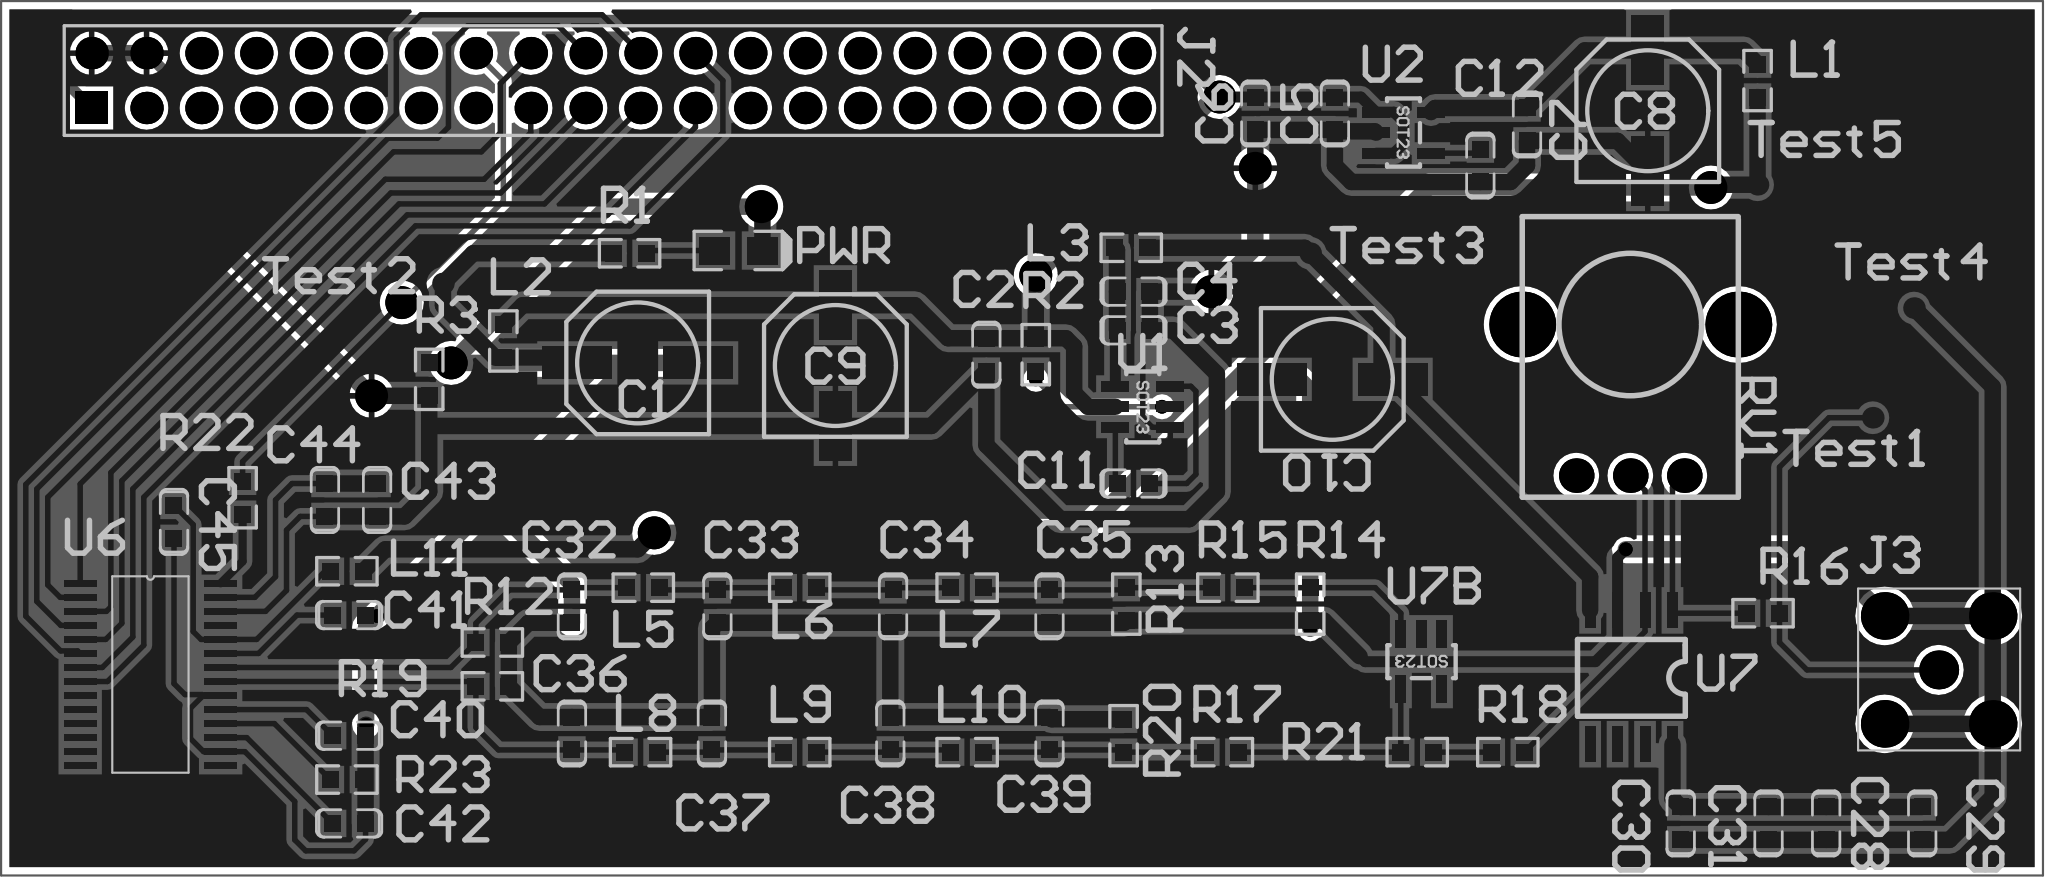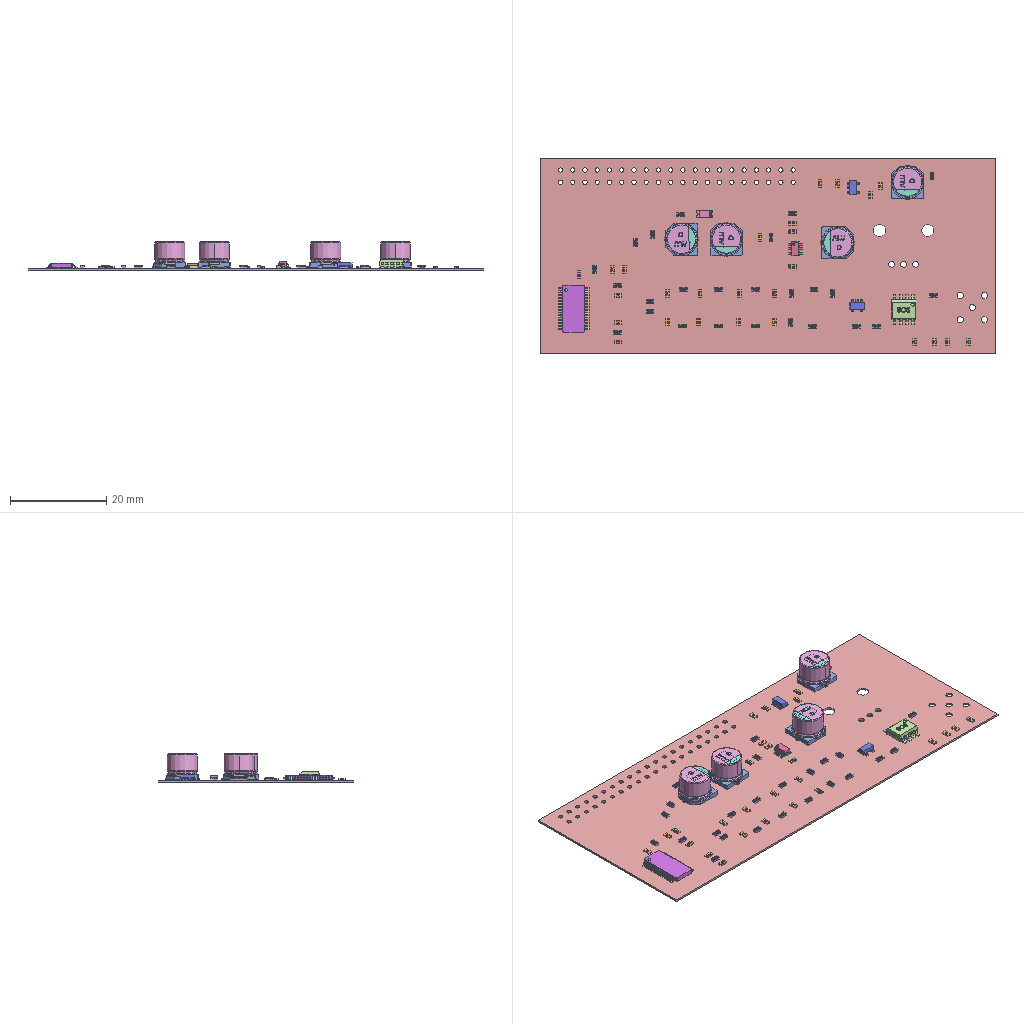Circuit board layout | Altium Designer | box 94.5 x 40.5 x 5.8 mm
Layer stack:
# Altium Designer layer stack of  (unit mm; dielectric type: 0 none, 1 core, 2 prepreg, 3 surface material)
index,name,kind,layer,copper_thickness_mm,dielectric_type,dielectric_thickness_mm,dielectric_material,dielectric_constant
0,Top Paste,other,,,,,,
1,Top Overlay,other,,,,,,
2,Top Solder,dielectric,,,3,0.0102,Solder Resist,3.5
3,Top Layer,copper,Top Layer,0.0356,,,,
4,Dielectric 1,dielectric,,,0,0.32,FR-4,4.8
5,Bottom Layer,copper,Bottom Layer,0.0356,,,,
6,Bottom Solder,dielectric,,,3,0.0102,Solder Resist,3.5
7,Bottom Overlay,other,,,,,,
8,Bottom Paste,other,,,,,,
# drill layer pairs: low layer,high layer
drill_pair,Top Layer,Bottom Layer
Part placement:
Designator,Comment,Layer,Footprint,Center-X(mm),Center-Y(mm),Rotation
C1,470uF/10V,TopLayer,CS_6.3mm*5.4mm,62.481,81.661,0
C2,3.3uF,TopLayer,CAP-SMD-0603,78.613,82.042,90
C3,3.3uF,TopLayer,CAP-SMD-0603,85.421,83.17,0
C4,10uF,TopLayer,CAP-SMD-0603,85.421,84.963,360
C9,470uF/10V,TopLayer,CS_6.3mm*5.4mm,71.628,81.537,270
C10,4700uF/10V,TopLayer,CS_6.3mm*5.4mm,94.618,80.899,180
C11,3.3uF,TopLayer,CAP-SMD-0603,85.421,76.073,180
C28,10uF,TopLayer,CAP-SMD-0603,117.475,60.325,90
C29,104,TopLayer,CAP-SMD-0603,121.92,60.325,90
C30,10uF,TopLayer,CAP-SMD-0603,110.744,60.325,90
C31,104,TopLayer,CAP-SMD-0603,114.808,60.325,90
C32,100pF,TopLayer,CAP-SMD-0603,59.436,70.383,90
C33,NF,TopLayer,CAP-SMD-0603,66.167,70.383,90
C34,NF,TopLayer,CAP-SMD-0603,74.295,70.383,90
C35,NF,TopLayer,CAP-SMD-0603,81.534,70.383,90
C36,100pF,TopLayer,CAP-SMD-0603,59.436,64.491,270
C37,NF,TopLayer,CAP-SMD-0603,65.913,64.491,270
C38,100pF,TopLayer,CAP-SMD-0603,74.168,64.491,270
C39,NF,TopLayer,CAP-SMD-0603,81.534,64.491,270
C40,104,TopLayer,CAP-SMD-0603,49.124,64.389,180
C41,104,TopLayer,CAP-SMD-0603,49.124,69.977,360
C42,104,TopLayer,CAP-SMD-0603,49.124,60.325,360
C43,104,TopLayer,CAP-SMD-0603,50.419,75.311,90
C44,1uF,TopLayer,CAP-SMD-0603,48.006,75.311,90
C45,104,TopLayer,CAP-SMD-0603,41.021,74.295,270
J3,SMA-KWE,TopLayer,SMA-KHD,122.682,67.437,180
L2,22uH,TopLayer,RES-SMD-0603,56.261,82.677,90
L3,22uH,TopLayer,RES-SMD-0603,85.319,86.995,180
L5,470nH,TopLayer,RES-SMD-0603,62.738,71.247,180
L6,820nH,TopLayer,RES-SMD-0603,69.977,71.247,180
L7,470nH,TopLayer,RES-SMD-0603,77.724,71.247,180
L8,470nH,TopLayer,RES-SMD-0603,62.611,63.627,180
L9,820nH,TopLayer,RES-SMD-0603,69.977,63.627,180
L10,470nH,TopLayer,RES-SMD-0603,77.724,63.627,180
L11,22uH,TopLayer,RES-SMD-0603,49.022,72.009,360
R2,10K,TopLayer,RES-SMD-0603,80.899,82.042,270
R3,0R,TopLayer,RES-SMD-0603,52.832,80.899,90
R12,100R,TopLayer,RES-SMD-0603,55.753,68.707,360
R13,100R,TopLayer,RES-SMD-0603,85.09,70.485,270
R14,1K,TopLayer,RES-SMD-0603,93.599,70.485,270
R15,1K,TopLayer,RES-SMD-0603,89.789,71.247,360
R16,51R,TopLayer,RES-SMD-0603,114.554,70.064,360
R17,1K,TopLayer,RES-SMD-0603,89.535,63.627,360
R18,1K,TopLayer,RES-SMD-0603,102.743,63.627,360
R19,100R,TopLayer,RES-SMD-0603,55.753,66.675,360
R20,100R,TopLayer,RES-SMD-0603,84.963,64.389,90
R21,1K,TopLayer,RES-SMD-0603,98.552,63.627,360
R22,33R,TopLayer,RES-SMD-0603,44.196,75.413,270
R23,2K,TopLayer,RES-SMD-0603,49.022,62.357,180
RV1,10K,TopLayer,RES-RV09,108.411,79.939,360
Test1,Test,TopLayer,Test,119.634,79.121,90
Test2,Test,TopLayer,Test,53.467,85.344,360
Test3,Test,TopLayer,Test,93.599,86.741,90
U1,SGM3204,TopLayer,SOT-23-6,85.852,79.629,0
U6,3PD9708E,TopLayer,TSSOP-28-NoHot,39.93,67.224,0
U7B,LMH6643,TopLayer,SOT-23-5,98.745,67.818,270
U7,LMH6643,TopLayer,SOIC-8,108.458,67.094,270
C5,10uF,TopLayer,CAP-SMD-0603,94.742,93.218,90
C6,104,TopLayer,CAP-SMD-0603,91.059,93.218,90
C7,104,TopLayer,CAP-SMD-0603,103.632,92.71,90
C8,470uF/10V,TopLayer,CS_6.3mm*5.4mm,109.22,93.342,270
C12,233,TopLayer,CAP-SMD-0603,101.473,90.805,90
J2,Header-HS_AD_DA-2*20-2.54mm,TopLayer,HEADER-HS-AD-DA-2*20-2.54MM,61.341,94.742,360
L1,22uH,TopLayer,RES-SMD-0603,114.3,94.742,90
PWR,LED-0805,TopLayer,LED-SMD-0805,67.145,86.868,360
R1,510R,TopLayer,RES-SMD-0603,62.103,86.741,360
Test4,Test,TopLayer,Test,121.539,84.201,90
Test5,Test,TopLayer,Test,114.3,89.916,90
U2,RT9193-3.3,TopLayer,SOT-23-5,97.917,92.329,360
Pad and via stacks:
# Altium Designer via and pad stacks of  (unit mm). Each distinct definition once, with the count of objects using it.
# via: kind,start_layer,end_layer,hole_mm,diameter_mm,mode(0 simple;1 top-mid-bottom;2 full stack),diameter_per_layer,count,example_net
# pad: kind,layer,hole_mm,hole_type(0 round;1 square;2 slot),plating,top_size,top_shape(1 round;2 rect;3 octagon;9 rounded rect),mid_size,bottom_size,mode,footprint,size_per_layer,count,example
pad,Top Layer,0,0,plated,1x1,1,1x1,1x1,0,Test,,5,Test2.1
pad,Top Layer,0,0,plated,3.2x1.5,2,3.2x1.5,3.2x1.5,0,CS 6.3mm*5.4mm,,8,C1.1
pad,Top Layer,0,0,plated,0.762x0.762,2,0.762x0.762,0.762x0.762,0,RES-SMD-0603,,50,L3.2
pad,Top Layer,0,0,plated,0.762x0.762,2,0.762x0.762,0.762x0.762,0,CAP-SMD-0603,,52,C30.2
pad,Top Layer,0,0,plated,0.508x1.27,2,0.508x1.27,0.508x1.27,0,SOT-23-5,,10,U7B.4
pad,Top Layer,0,0,plated,1.5x0.3,2,1.5x0.3,1.5x0.3,0,TSSOP-28-NoHot,,28,U6.15
pad,Top Layer,0,0,plated,0.5x1.65,2,0.5x1.65,0.5x1.65,0,SOIC-8,,8,U7.1
pad,Top Layer,0,0,plated,0.508x1.27,2,0.508x1.27,0.508x1.27,0,SOT-23-6,,6,U1.4
pad,Top Layer,0,0,plated,1.4x1.27,2,1.4x1.27,1.4x1.27,0,LED-SMD-0805,,2,PWR.2
pad,Multi-Layer,1.3,0,plated,1.8x1.8,1,1.8x1.8,1.8x1.8,0,SMA-KHD,,1,J3.1
pad,Multi-Layer,1.3,0,plated,2.2x2.2,1,2.2x2.2,2.2x2.2,0,SMA-KHD,,4,J3.5
pad,Multi-Layer,1.2,0,plated,1.6x1.6,1,1.6x1.6,1.6x1.6,0,RES-RV09,,3,RV1.1
pad,Multi-Layer,2.5,0,plated,3.048x3.048,1,3.048x3.048,3.048x3.048,0,RES-RV09,,2,RV1.0
pad,Multi-Layer,0.9,0,plated,1.5x1.5,2,1.5x1.5,1.5x1.5,0,HEADER-HS-AD-DA-2*20-2.54MM,,1,J2.1
pad,Multi-Layer,0.9,0,plated,1.5x1.5,1,1.5x1.5,1.5x1.5,0,HEADER-HS-AD-DA-2*20-2.54MM,,39,J2.2
via,Top Layer,Bottom Layer,0.381,0.635,0,,9,AGND
via,Top Layer,Bottom Layer,0.762,1.524,0,,10,GND
Copper pours:
name,layer,net,type(0 solid;1 hatched;2 none)
Top Layer-No Net,Top Layer,GND,0
Top Layer-No Net,Bottom Layer,GND,0
Design rules, without the lines most boards share:
# Altium Designer design rules of  (exported by Altium Designer, unit mm)
# columns: name | kind | enabled | priority | scope1 | scope2 | descriptor | typed fields (field=value)
Clearance | 0 | enabled | 1 | All | All | Clearance Constraint (Gap=10mil) (All),(All) | gap=0.254
PlaneConnect | 6 | enabled | 1 | All | All | Power Plane Connect Rule(Relief Connect )(Expansion=20mil) (Conductor Width=10mil) (Air Gap=10mil) (Entries=4) (All) | relief_conductor_width=0.254 relief_entries=4 relief_expansion=0.508
PolygonConnect | 20 | enabled | 1 | All | All | Polygon Connect Rule(Relief Connect )(Conductor Width=10mil) (Relief Angle=90 Angle) (Entries=4) (Air Gap Width=10mil) (All),(All) | connect_style(0=relief,1=direct,2=none)=0 relief_conductor_width=0.254 relief_entries=4
Width | 2 | enabled | 1 | All | All | Width Constraint (Min=10mil) (Max=30mil) (Preferred=10mil) (All) |
RoutingVias | 11 | enabled | 1 | All | All | Routing Via (MinHoleWidth=28mil) (MaxHoleWidth=28mil) (PreferredHoleWidth=28mil) (MinWidth=50mil) (MaxWidth=50mil) (PreferedWidth=50mil) (All) | via_min_hole=0.7112 via_max_hole=0.7112 via_preferred_diameter=1.27 via_preferred_hole=0.7112
PasteMaskExpansion | 14 | enabled | 1 | All | All | Paste Mask Expansion (Expansion =0mil) (All) | expansion=0
SolderMaskExpansion | 13 | enabled | 1 | All | All | Solder Mask Expansion (Expansion =4mil) (All) | expansion=0.1016
DiffPairsRouting | 51 | enabled | 1 | All | All | Differential Pairs Uncoupled Length using the Gap Constraints (Min=10mil) (Max=10mil) (Prefered=10mil)  and Width Constraints (Min=15mil) (Max=15mil) (Prefered=15mil) (All) |
HoleToHoleClearance | 52 | enabled | 1 | All | All | Hole To Hole Clearance (Gap=10mil) (All),(All) | gap=0.254
MinimumSolderMaskSliver | 53 | enabled | 1 | All | All | Minimum Solder Mask Sliver (Gap=0mil) (All),(All) |
SilkToSolderMaskClearance | 54 | enabled | 1 | IsPad | All | Silk To Solder Mask (Clearance=0mil) (IsPad),(All) |
SilkToSilkClearance | 55 | enabled | 1 | All | All | Silk to Silk (Clearance=0mil) (All),(All) |
Classes set for this board:
# Altium Designer classes of  (member kind: 0 net, 1 component, 2 from-to, 3 pad, 4 layer, 5 differential pair, 6 design channel, 7 polygon, 8 structure, 9 xSignal)
# columns: class name | member kind | superclass | members
DAC | 1 | no | C1; C2; C3; C4; C9; C10; C11; C28; C29; C30; C31; C32; C33; C34; C35; C36; C37; C38; C39; C40; C41; C42; C43; C44; C45; J3; L2; L3; L5; L6; L7; L8; L9; L10; L11; R2; R3; R12; R13; R14; R15; R16; R17; R18; R19; R20; R21; R22; R23; RV1; Test1; Test2; Test3; U1; U7; U7B; C5; C6; C7; C8; C12; J2; L1; PWR; R1; Test4; Test5; U2; U6;